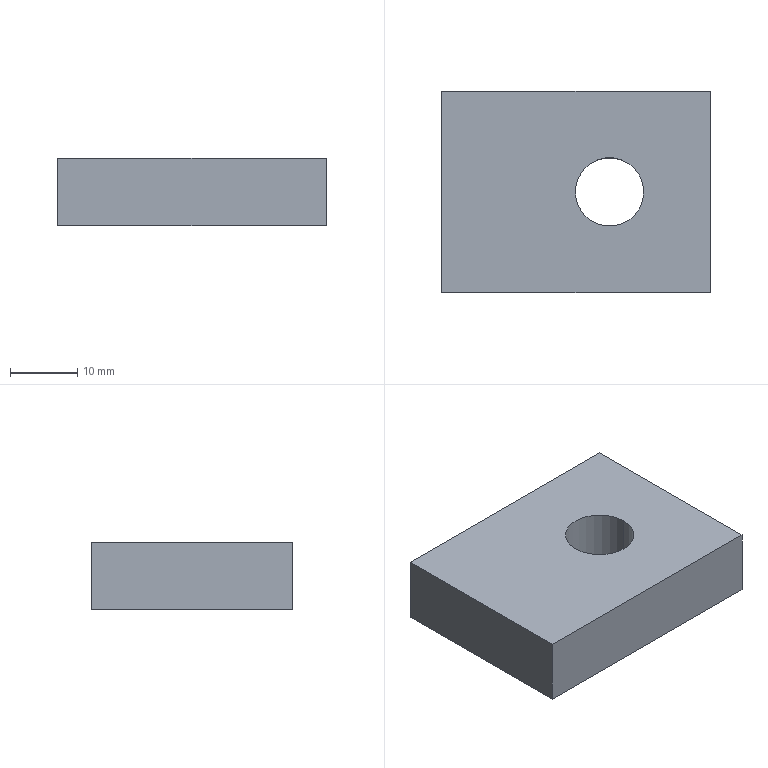Part | SolidWorks | features 3DProfileFeature 1, Extrusion 1, HoleWzd 1 | 1 solid | 8 faces | box 40 x 30 x 10 mm | volume 11183 mm3 | plane 6 | cylinder 2 | commonest cylinder face diameters 10.2 x2
STEP:
#1=CARTESIAN_POINT('',(10.1,0.,10.));
#2=VERTEX_POINT('',#1);
#3=CARTESIAN_POINT('',(-0.1,0.,10.));
#4=VERTEX_POINT('',#3);
#5=CARTESIAN_POINT('',(5.,0.,10.));
#6=DIRECTION('',(0.,0.,-1.));
#7=DIRECTION('',(-1.,0.,0.));
#8=AXIS2_PLACEMENT_3D('',#5,#6,#7);
#9=CIRCLE('',#8,5.1);
#10=EDGE_CURVE('',#2,#4,#9,.T.);
#11=ORIENTED_EDGE('',*,*,#10,.F.);
#12=CARTESIAN_POINT('',(10.1,0.,0.));
#13=VERTEX_POINT('',#12);
#14=CARTESIAN_POINT('',(10.1,0.,0.));
#15=DIRECTION('',(0.,0.,-1.));
#16=VECTOR('',#15,1000.);
#17=LINE('',#14,#16);
#18=EDGE_CURVE('',#2,#13,#17,.T.);
#19=ORIENTED_EDGE('',*,*,#18,.T.);
#20=CARTESIAN_POINT('',(-0.1,0.,0.));
#21=VERTEX_POINT('',#20);
#22=CARTESIAN_POINT('',(5.,0.,0.));
#23=DIRECTION('',(0.,0.,-1.));
#24=DIRECTION('',(-1.,0.,0.));
#25=AXIS2_PLACEMENT_3D('',#22,#23,#24);
#26=CIRCLE('',#25,5.1);
#27=EDGE_CURVE('',#13,#21,#26,.T.);
#28=ORIENTED_EDGE('',*,*,#27,.T.);
#29=CARTESIAN_POINT('',(-0.1,0.,0.));
#30=DIRECTION('',(0.,0.,-1.));
#31=VECTOR('',#30,1000.);
#32=LINE('',#29,#31);
#33=EDGE_CURVE('',#4,#21,#32,.T.);
#34=ORIENTED_EDGE('',*,*,#33,.F.);
#35=EDGE_LOOP('',(#11,#19,#28,#34));
#36=FACE_OUTER_BOUND('',#35,.T.);
#37=CARTESIAN_POINT('',(5.,0.,0.));
#38=DIRECTION('',(0.,0.,-1.));
#39=DIRECTION('',(-1.,0.,0.));
#40=AXIS2_PLACEMENT_3D('',#37,#38,#39);
#41=CYLINDRICAL_SURFACE('',#40,5.1);
#42=ADVANCED_FACE('',(#36),#41,.F.);
#43=CARTESIAN_POINT('',(5.,0.,10.));
#44=DIRECTION('',(0.,0.,-1.));
#45=DIRECTION('',(-1.,0.,0.));
#46=AXIS2_PLACEMENT_3D('',#43,#44,#45);
#47=CIRCLE('',#46,5.1);
#48=EDGE_CURVE('',#4,#2,#47,.T.);
#49=ORIENTED_EDGE('',*,*,#48,.T.);
#50=ORIENTED_EDGE('',*,*,#10,.T.);
#51=EDGE_LOOP('',(#49,#50));
#52=FACE_BOUND('',#51,.T.);
#53=CARTESIAN_POINT('',(20.,-15.,10.));
#54=VERTEX_POINT('',#53);
#55=CARTESIAN_POINT('',(20.,15.,10.));
#56=VERTEX_POINT('',#55);
#57=CARTESIAN_POINT('',(20.,-15.,10.));
#58=DIRECTION('',(0.,1.,0.));
#59=VECTOR('',#58,1000.);
#60=LINE('',#57,#59);
#61=EDGE_CURVE('',#54,#56,#60,.T.);
#62=ORIENTED_EDGE('',*,*,#61,.T.);
#63=CARTESIAN_POINT('',(-20.,15.,10.));
#64=VERTEX_POINT('',#63);
#65=CARTESIAN_POINT('',(-20.,15.,10.));
#66=DIRECTION('',(-1.,0.,0.));
#67=VECTOR('',#66,1000.);
#68=LINE('',#65,#67);
#69=EDGE_CURVE('',#56,#64,#68,.T.);
#70=ORIENTED_EDGE('',*,*,#69,.T.);
#71=CARTESIAN_POINT('',(-20.,-15.,10.));
#72=VERTEX_POINT('',#71);
#73=CARTESIAN_POINT('',(-20.,-15.,10.));
#74=DIRECTION('',(0.,-1.,0.));
#75=VECTOR('',#74,1000.);
#76=LINE('',#73,#75);
#77=EDGE_CURVE('',#64,#72,#76,.T.);
#78=ORIENTED_EDGE('',*,*,#77,.T.);
#79=CARTESIAN_POINT('',(-20.,-15.,10.));
#80=DIRECTION('',(1.,0.,0.));
#81=VECTOR('',#80,1000.);
#82=LINE('',#79,#81);
#83=EDGE_CURVE('',#72,#54,#82,.T.);
#84=ORIENTED_EDGE('',*,*,#83,.T.);
#85=EDGE_LOOP('',(#62,#70,#78,#84));
#86=FACE_OUTER_BOUND('',#85,.T.);
#87=CARTESIAN_POINT('',(0.,0.,10.));
#88=DIRECTION('',(0.,0.,-1.));
#89=DIRECTION('',(-1.,0.,0.));
#90=AXIS2_PLACEMENT_3D('',#87,#88,#89);
#91=PLANE('',#90);
#92=ADVANCED_FACE('',(#52,#86),#91,.F.);
#93=CARTESIAN_POINT('',(5.,0.,0.));
#94=DIRECTION('',(0.,0.,-1.));
#95=DIRECTION('',(-1.,0.,0.));
#96=AXIS2_PLACEMENT_3D('',#93,#94,#95);
#97=CIRCLE('',#96,5.1);
#98=EDGE_CURVE('',#21,#13,#97,.T.);
#99=ORIENTED_EDGE('',*,*,#98,.F.);
#100=ORIENTED_EDGE('',*,*,#27,.F.);
#101=EDGE_LOOP('',(#99,#100));
#102=FACE_BOUND('',#101,.T.);
#103=CARTESIAN_POINT('',(20.,-15.,0.));
#104=VERTEX_POINT('',#103);
#105=CARTESIAN_POINT('',(20.,15.,0.));
#106=VERTEX_POINT('',#105);
#107=CARTESIAN_POINT('',(20.,-15.,0.));
#108=DIRECTION('',(0.,1.,0.));
#109=VECTOR('',#108,1000.);
#110=LINE('',#107,#109);
#111=EDGE_CURVE('',#104,#106,#110,.T.);
#112=ORIENTED_EDGE('',*,*,#111,.F.);
#113=CARTESIAN_POINT('',(-20.,-15.,0.));
#114=VERTEX_POINT('',#113);
#115=CARTESIAN_POINT('',(-20.,-15.,0.));
#116=DIRECTION('',(1.,0.,0.));
#117=VECTOR('',#116,1000.);
#118=LINE('',#115,#117);
#119=EDGE_CURVE('',#114,#104,#118,.T.);
#120=ORIENTED_EDGE('',*,*,#119,.F.);
#121=CARTESIAN_POINT('',(-20.,15.,0.));
#122=VERTEX_POINT('',#121);
#123=CARTESIAN_POINT('',(-20.,-15.,0.));
#124=DIRECTION('',(0.,-1.,0.));
#125=VECTOR('',#124,1000.);
#126=LINE('',#123,#125);
#127=EDGE_CURVE('',#122,#114,#126,.T.);
#128=ORIENTED_EDGE('',*,*,#127,.F.);
#129=CARTESIAN_POINT('',(-20.,15.,0.));
#130=DIRECTION('',(-1.,0.,0.));
#131=VECTOR('',#130,1000.);
#132=LINE('',#129,#131);
#133=EDGE_CURVE('',#106,#122,#132,.T.);
#134=ORIENTED_EDGE('',*,*,#133,.F.);
#135=EDGE_LOOP('',(#112,#120,#128,#134));
#136=FACE_OUTER_BOUND('',#135,.T.);
#137=CARTESIAN_POINT('',(0.,0.,0.));
#138=DIRECTION('',(0.,0.,-1.));
#139=DIRECTION('',(-1.,0.,0.));
#140=AXIS2_PLACEMENT_3D('',#137,#138,#139);
#141=PLANE('',#140);
#142=ADVANCED_FACE('',(#102,#136),#141,.T.);
#143=ORIENTED_EDGE('',*,*,#111,.T.);
#144=CARTESIAN_POINT('',(20.,15.,10.));
#145=DIRECTION('',(0.,0.,-1.));
#146=VECTOR('',#145,1000.);
#147=LINE('',#144,#146);
#148=EDGE_CURVE('',#56,#106,#147,.T.);
#149=ORIENTED_EDGE('',*,*,#148,.F.);
#150=ORIENTED_EDGE('',*,*,#61,.F.);
#151=CARTESIAN_POINT('',(20.,-15.,10.));
#152=DIRECTION('',(0.,0.,-1.));
#153=VECTOR('',#152,1000.);
#154=LINE('',#151,#153);
#155=EDGE_CURVE('',#54,#104,#154,.T.);
#156=ORIENTED_EDGE('',*,*,#155,.T.);
#157=EDGE_LOOP('',(#143,#149,#150,#156));
#158=FACE_OUTER_BOUND('',#157,.T.);
#159=CARTESIAN_POINT('',(20.,-15.,10.));
#160=DIRECTION('',(-1.,0.,0.));
#161=DIRECTION('',(0.,0.,1.));
#162=AXIS2_PLACEMENT_3D('',#159,#160,#161);
#163=PLANE('',#162);
#164=ADVANCED_FACE('',(#158),#163,.F.);
#165=ORIENTED_EDGE('',*,*,#133,.T.);
#166=CARTESIAN_POINT('',(-20.,15.,10.));
#167=DIRECTION('',(0.,0.,-1.));
#168=VECTOR('',#167,1000.);
#169=LINE('',#166,#168);
#170=EDGE_CURVE('',#64,#122,#169,.T.);
#171=ORIENTED_EDGE('',*,*,#170,.F.);
#172=ORIENTED_EDGE('',*,*,#69,.F.);
#173=ORIENTED_EDGE('',*,*,#148,.T.);
#174=EDGE_LOOP('',(#165,#171,#172,#173));
#175=FACE_OUTER_BOUND('',#174,.T.);
#176=CARTESIAN_POINT('',(-20.,15.,10.));
#177=DIRECTION('',(0.,-1.,0.));
#178=DIRECTION('',(0.,0.,-1.));
#179=AXIS2_PLACEMENT_3D('',#176,#177,#178);
#180=PLANE('',#179);
#181=ADVANCED_FACE('',(#175),#180,.F.);
#182=ORIENTED_EDGE('',*,*,#127,.T.);
#183=CARTESIAN_POINT('',(-20.,-15.,10.));
#184=DIRECTION('',(0.,0.,-1.));
#185=VECTOR('',#184,1000.);
#186=LINE('',#183,#185);
#187=EDGE_CURVE('',#72,#114,#186,.T.);
#188=ORIENTED_EDGE('',*,*,#187,.F.);
#189=ORIENTED_EDGE('',*,*,#77,.F.);
#190=ORIENTED_EDGE('',*,*,#170,.T.);
#191=EDGE_LOOP('',(#182,#188,#189,#190));
#192=FACE_OUTER_BOUND('',#191,.T.);
#193=CARTESIAN_POINT('',(-20.,-15.,10.));
#194=DIRECTION('',(1.,0.,0.));
#195=DIRECTION('',(0.,0.,-1.));
#196=AXIS2_PLACEMENT_3D('',#193,#194,#195);
#197=PLANE('',#196);
#198=ADVANCED_FACE('',(#192),#197,.F.);
#199=ORIENTED_EDGE('',*,*,#119,.T.);
#200=ORIENTED_EDGE('',*,*,#155,.F.);
#201=ORIENTED_EDGE('',*,*,#83,.F.);
#202=ORIENTED_EDGE('',*,*,#187,.T.);
#203=EDGE_LOOP('',(#199,#200,#201,#202));
#204=FACE_OUTER_BOUND('',#203,.T.);
#205=CARTESIAN_POINT('',(-20.,-15.,10.));
#206=DIRECTION('',(0.,1.,0.));
#207=DIRECTION('',(0.,0.,1.));
#208=AXIS2_PLACEMENT_3D('',#205,#206,#207);
#209=PLANE('',#208);
#210=ADVANCED_FACE('',(#204),#209,.F.);
#211=ORIENTED_EDGE('',*,*,#18,.F.);
#212=ORIENTED_EDGE('',*,*,#48,.F.);
#213=ORIENTED_EDGE('',*,*,#33,.T.);
#214=ORIENTED_EDGE('',*,*,#98,.T.);
#215=EDGE_LOOP('',(#211,#212,#213,#214));
#216=FACE_OUTER_BOUND('',#215,.T.);
#217=CARTESIAN_POINT('',(5.,0.,0.));
#218=DIRECTION('',(0.,0.,-1.));
#219=DIRECTION('',(-1.,0.,0.));
#220=AXIS2_PLACEMENT_3D('',#217,#218,#219);
#221=CYLINDRICAL_SURFACE('',#220,5.1);
#222=ADVANCED_FACE('',(#216),#221,.F.);
#223=CLOSED_SHELL('',(#42,#92,#142,#164,#181,#198,#210,#222));
#224=MANIFOLD_SOLID_BREP('',#223);
#225=CARTESIAN_POINT('',(0.,0.,0.));
#226=DIRECTION('',(0.,0.,1.));
#227=DIRECTION('',(1.,0.,0.));
#228=AXIS2_PLACEMENT_3D('',#225,#226,#227);
#229=(LENGTH_UNIT()NAMED_UNIT(*)SI_UNIT(.MILLI.,.METRE.));
#230=UNCERTAINTY_MEASURE_WITH_UNIT(LENGTH_MEASURE(0.00001),#229,'','');
#231=(NAMED_UNIT(*)PLANE_ANGLE_UNIT()SI_UNIT($,.RADIAN.));
#232=(NAMED_UNIT(*)SI_UNIT($,.STERADIAN.)SOLID_ANGLE_UNIT());
#233=(GEOMETRIC_REPRESENTATION_CONTEXT(3)GLOBAL_UNCERTAINTY_ASSIGNED_CONTEXT((#230))GLOBAL_UNIT_ASSIGNED_CONTEXT((#229,#231,#232))REPRESENTATION_CONTEXT('',''));
#234=ADVANCED_BREP_SHAPE_REPRESENTATION('',(#224,#228),#233);